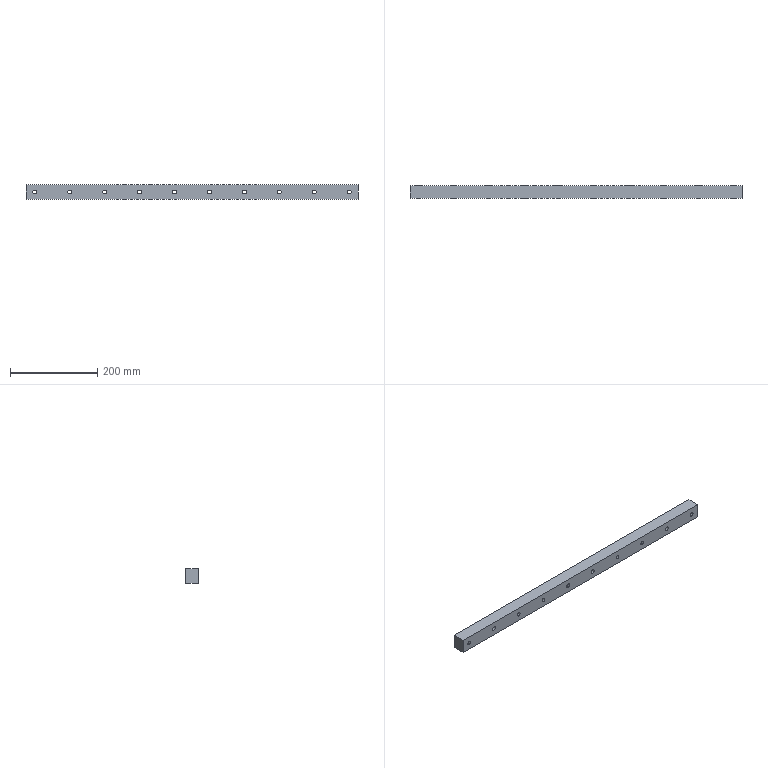Part | SolidWorks | features Cut 2, Extrusion 1, LPattern 1 | 1 solid | 56 faces | box 760 x 29 x 34 mm | volume 720073 mm3 | cylinder 40 | plane 16 | commonest cylinder face diameters 9 x20 14 x20